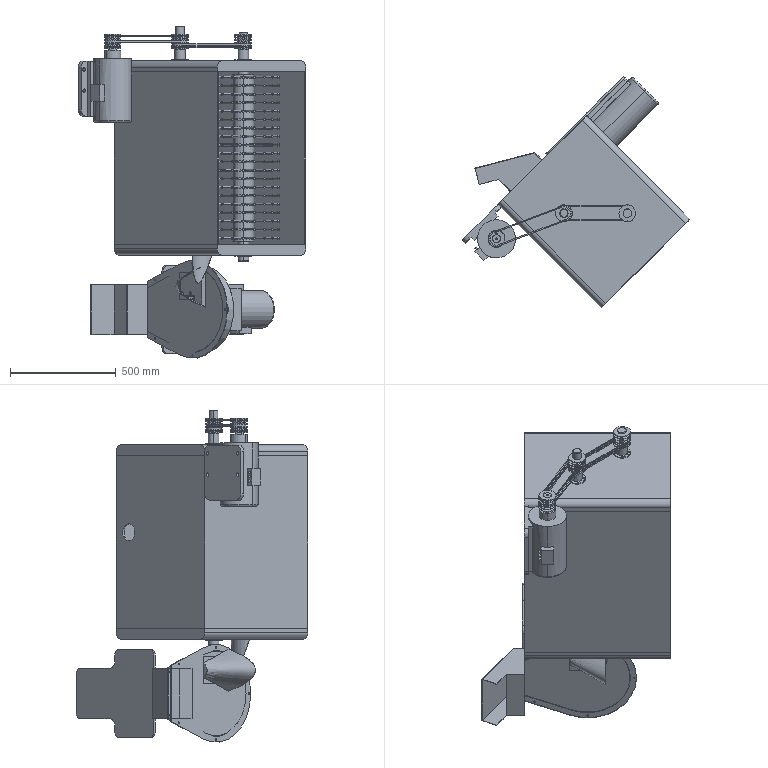Part | SolidWorks | features AEMSimFeature 1 | 940 solids | 4719 faces | volume 106824428 mm3 | cylinder 2139 | plane 2026 | sphere 352 | cone 126 | torus 66 | spline 10 | commonest cylinder face diameters 10 x1648 7 x68 60 x64 80 x48 6 x29 16 x20